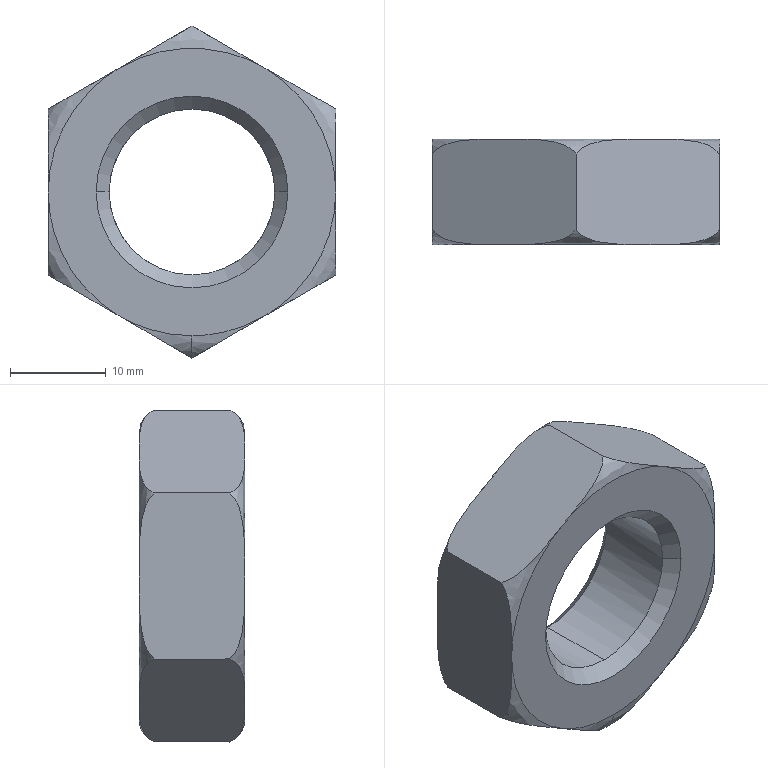Part | SolidWorks | features BaseBody 1 | 1 solid | 28 faces | box 30 x 11 x 34.641 mm | volume 5861 mm3 | spline 14 | plane 8 | cone 4 | cylinder 2 | commonest cylinder face diameters 17.294 x2